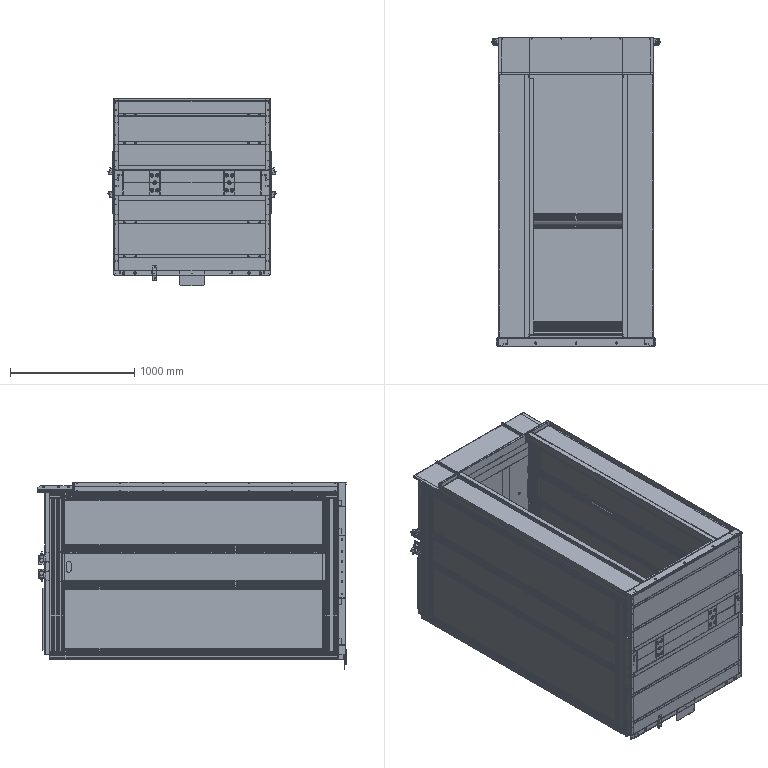Part | SolidWorks | 333 solids | 11496 faces | volume 297784141 mm3 | plane 7318 | cylinder 3914 | cone 264 | commonest cylinder face diameters 6 x378 10 x333 11 x315 0.4 x274 8.5 x220 1.1 x216